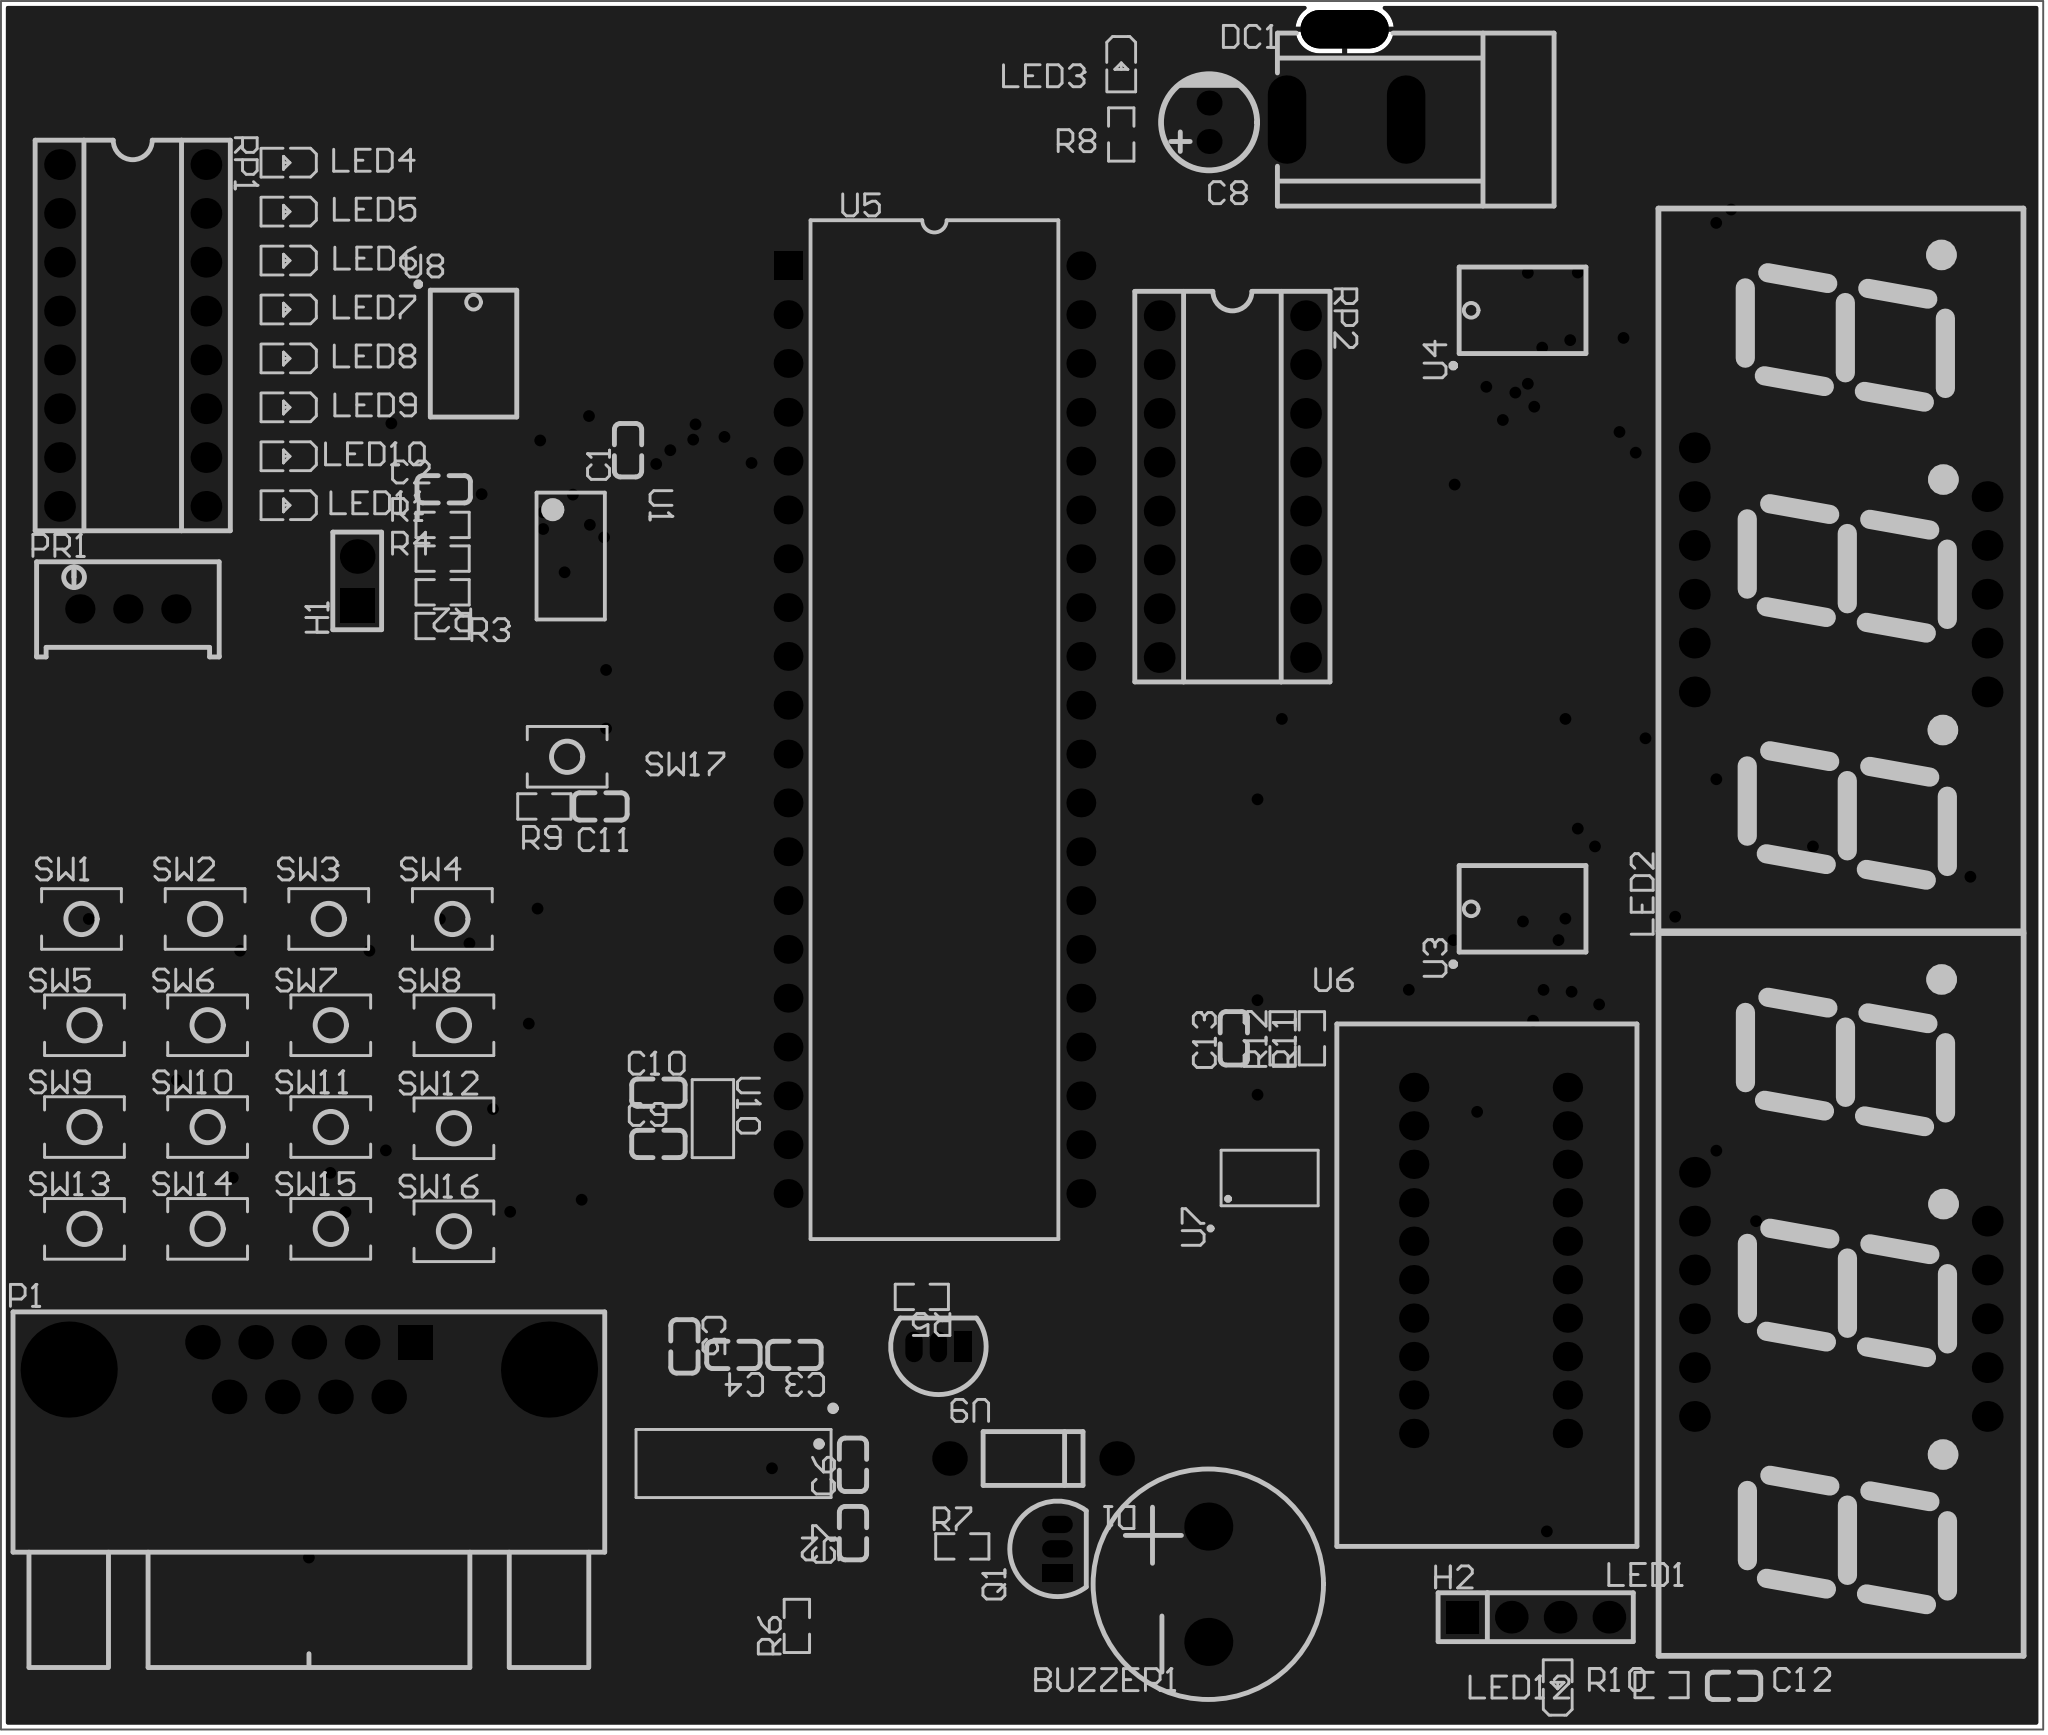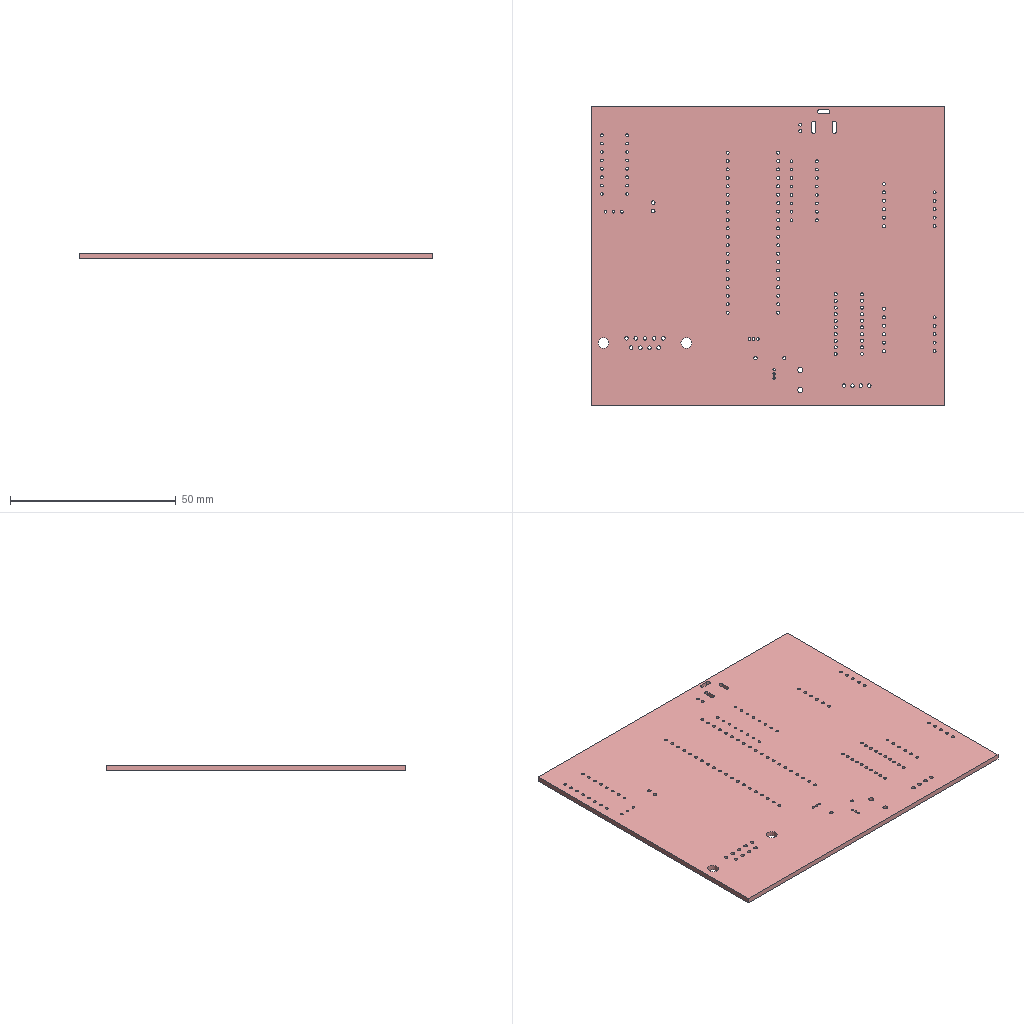Circuit board layout | Altium Designer | box 106.3 x 89.9 x 1.6 mm
Layer stack:
# Altium Designer layer stack of  (unit mm; dielectric type: 0 none, 1 core, 2 prepreg, 3 surface material)
index,name,kind,layer,copper_thickness_mm,dielectric_type,dielectric_thickness_mm,dielectric_material,dielectric_constant
0,Top Paste Mask Layer,other,,,,,,
1,Top Silkscreen Layer,other,,,,,,
2,Top Solder Mask Layer,dielectric,,,3,0.01,,3.3
3,Top Layer,copper,Top Layer,0.035,,,,
4,Dielectric1,dielectric,,,3,1.51,FR4,4.5
5,Bottom Layer,copper,Bottom Layer,0.035,,,,
6,Bottom Solder Mask Layer,dielectric,,,3,0.01,,3.3
7,Bottom Silkscreen Layer,other,,,,,,
8,Bottom Paste Mask Layer,other,,,,,,
# drill layer pairs: low layer,high layer
drill_pair,Top Layer,Bottom Layer
Part placement:
Designator,Comment,Layer,Footprint,Center-X(mm),Center-Y(mm),Rotation
BUZZER1,buzzer,TopLayer,BUZ-TH_BD12.0-P6.00-D0.9-RD,147.931,100.139,90
C1,104,TopLayer,C0603,117.729,159.131,90
C2,104,TopLayer,C0603,108.133,157.099,0
C3,104,TopLayer,C0603,126.389,112.069,180
C4,104,TopLayer,C0603,123.214,112.069,180
C5,104,TopLayer,C0603,120.664,112.512,270
C6,104,TopLayer,C0603,129.437,106.354,90
C7,104,TopLayer,C0603,129.437,102.798,90
C8,100uF,TopLayer,CAP-TH_BD5.0-P2.00-D0.8-FD-10UF50VC110GL,147.973,176.19,90
C9,20PF,TopLayer,C0603,119.31,123.044,0
C10,20PF,TopLayer,C0603,119.31,125.711,0
C11,10uF,TopLayer,C0603,116.293,140.6,0
C12,104,TopLayer,C0603,175.297,94.854,0
C13,104,TopLayer,C0603,149.26,128.538,90
D1,,TopLayer,DO_1N4007,138.811,106.68,180
DC1,,TopLayer,DC-005_2.5,155.129,178.682,0
H1,,TopLayer,HDR-TH_2P-P2.54-V-M-1,103.632,152.333,90
H2,,TopLayer,HDR-TH_4P-P2.54-V-M,164.973,98.425,0
LED1,3631BS,TopLayer,LED-SEG-TH_11P-L37.5-W19.0-P2.54-LS15.2-BL_1,180.856,115.219,90
LED2,3631BS,TopLayer,LED-SEG-TH_11P-L37.5-W19.0-P2.54-LS15.2-BL_1,180.848,152.908,90
LED3,,TopLayer,LED_0603,143.393,179.162,270
LED4,,TopLayer,LED_0603,100.015,174.095,180
LED5,,TopLayer,LED_0603,100.015,171.55,180
LED6,,TopLayer,LED_0603,100.015,169.004,180
LED7,,TopLayer,LED_0603,100.015,166.459,180
LED8,,TopLayer,LED_0603,100.015,163.913,180
LED9,,TopLayer,LED_0603,100.015,161.368,180
LED10,,TopLayer,LED_0603,100.015,158.822,180
LED11,,TopLayer,LED_0603,100.015,156.276,180
LED12,,TopLayer,LED_0603,166.124,94.818,90
P1,DB9FL,TopLayer,DB9-TH_DB9F,101.116,111.307,0
PR1,10kΩ,TopLayer,R_3296,91.694,150.876,0
Q1,,TopLayer,S8550P_TO-92,140.081,101.981,90
R1,10K,TopLayer,R0603,108.077,155.246,0
R2,1K,TopLayer,R0603,108.077,151.74,180
R3,1K,TopLayer,R0603,108.077,149.987,0
R4,510K,TopLayer,R0603,108.077,153.493,0
R5,4.7K,TopLayer,R0603,133.02,115.088,180
R6,0,TopLayer,R0603,126.516,97.972,90
R7,2K,TopLayer,R0603,135.128,102.108,0
R8,1K,TopLayer,R0603,143.401,175.555,270
R9,10K,TopLayer,R0603,113.372,140.6,0
R10,0,TopLayer,R0603,171.524,94.895,0
R11,4.7K,TopLayer,R0603,153.324,128.538,90
R12,4.7K,TopLayer,R0603,151.8,128.538,90
RP1,,TopLayer,DIP-16_L20.3-W10.2-P2.54-LS7.6-BL,91.948,165.1,270
RP2,,TopLayer,DIP-16_L20.3-W10.2-P2.54-LS7.6-BL,149.186,157.237,270
SW1,,TopLayer,Key_SMD_3x4x2,89.281,134.747,180
SW2,,TopLayer,Key_SMD_3x4x2,95.716,134.747,180
SW3,,TopLayer,Key_SMD_3x4x2,102.15,134.747,180
SW4,,TopLayer,Key_SMD_3x4x2,108.585,134.747,180
SW5,,TopLayer,Key_SMD_3x4x2,89.436,129.218,0
SW6,,TopLayer,Key_SMD_3x4x2,95.846,129.218,0
SW7,,TopLayer,Key_SMD_3x4x2,102.256,129.218,0
SW8,,TopLayer,Key_SMD_3x4x2,108.667,129.218,0
SW9,,TopLayer,Key_SMD_3x4x2,89.436,123.922,0
SW10,,TopLayer,Key_SMD_3x4x2,95.846,123.922,0
SW11,,TopLayer,Key_SMD_3x4x2,102.256,123.922,0
SW12,,TopLayer,Key_SMD_3x4x2,108.667,123.859,0
SW13,,TopLayer,Key_SMD_3x4x2,89.436,118.627,0
SW14,,TopLayer,Key_SMD_3x4x2,95.846,118.627,0
SW15,,TopLayer,Key_SMD_3x4x2,102.256,118.627,0
SW16,,TopLayer,Key_SMD_3x4x2,108.667,118.5,0
SW17,,TopLayer,Key_SMD_3x4x2,114.56,143.184,180
U1,ADC0804CN,TopLayer,ADC0804CN,114.745,153.626,270
U2,MAX232ESE,TopLayer,MAX232ESE,123.221,106.419,180
U3,MC74HC573DW,TopLayer,MC74HC573DW,164.239,135.295,90
U4,MC74HC573DW,TopLayer,MC74HC573DW,164.239,166.43,90
U5,P89C51RC2HBP,TopLayer,P89C51RC23N_01,133.678,144.595,270
U7,AT24C02,TopLayer,SOIC-8_L5.0-W4.0-P1.27-LS6.2-TL,151.124,121.272,90
U8,MC74HC573DW,TopLayer,MC74HC573DW,109.707,164.207,0
U9,DS18B20,TopLayer,TO-92-3_L4.9-W3.7-P1.27-L,133.884,112.489,180
U10,32768/10ppm/12.5pF,TopLayer,osc-smd_l3.2-w1.5,122.146,124.359,270
U6,DAC0832LCJ,TopLayer,DAC0832LCJ,162.624,116.984,0
Pad and via stacks:
# Altium Designer via and pad stacks of  (unit mm). Each distinct definition once, with the count of objects using it.
# via: kind,start_layer,end_layer,hole_mm,diameter_mm,mode(0 simple;1 top-mid-bottom;2 full stack),diameter_per_layer,count,example_net
# pad: kind,layer,hole_mm,hole_type(0 round;1 square;2 slot),plating,top_size,top_shape(1 round;2 rect;3 octagon;9 rounded rect),mid_size,bottom_size,mode,footprint,size_per_layer,count,example
pad,Multi-Layer,1.5,0,plated,2.5x2.5,1,2.5x2.5,2.5x2.5,0,BUZ-TH_BD12.0-P6.00-D0.9-RD,,2,BUZZER1.1
pad,Multi-Layer,0.9,0,plated,1.3x1.3,1,1.3x1.3,1.3x1.3,0,CAP-TH_BD5.0-P2.00-D0.8-FD-10UF50VC110GL,,2,C8.2
pad,Multi-Layer,1,0,plated,1.8x1.8,1,1.8x1.8,1.8x1.8,0,DO_1N4007,,2,D1.1
pad,Multi-Layer,1.2,2,plated,2x4.6,1,2x4.6,2x4.6,0,DC-005_2.5,,2,DC1.1
pad,Multi-Layer,1.2,2,plated,4.6x2,1,4.6x2,4.6x2,0,DC-005_2.5,,1,DC1.3
pad,Multi-Layer,1.1,0,plated,1.8x1.8,1,1.8x1.8,1.8x1.8,0,HDR-TH_2P-P2.54-V-M-1,,1,H1.2
pad,Multi-Layer,1.1,0,plated,1.8x1.8,2,1.8x1.8,1.8x1.8,0,HDR-TH_2P-P2.54-V-M-1,,1,H1.1
pad,Multi-Layer,1.1,0,plated,1.7x1.7,2,1.7x1.7,1.7x1.7,0,HDR-TH_4P-P2.54-V-M,,1,H2.1
pad,Multi-Layer,1.1,0,plated,1.7x1.7,1,1.7x1.7,1.7x1.7,0,HDR-TH_4P-P2.54-V-M,,3,H2.2
pad,Multi-Layer,0.9,0,plated,1.6x1.6,1,1.6x1.6,1.6x1.6,0,LED-SEG-TH_11P-L37.5-W19.0-P2.54-LS15.2-BL_1,,22,LED1.4
pad,Multi-Layer,3.25,0,plated,5x5,1,5x5,5x5,0,DB9-TH_DB9F,,2,P1.10
pad,Multi-Layer,1.1,0,plated,1.8x1.8,1,1.8x1.8,1.8x1.8,0,DB9-TH_DB9F,,8,P1.6
pad,Multi-Layer,1.1,0,plated,1.8x1.8,2,1.8x1.8,1.8x1.8,0,DB9-TH_DB9F,,1,P1.1
pad,Multi-Layer,0.762,0,plated,1.524x1.524,1,1.524x1.524,1.524x1.524,0,R_3296,,3,PR1.2
pad,Multi-Layer,0.7,0,plated,0.9x1.6,1,0.9x1.6,0.9x1.6,0,S8550P_TO-92,,2,Q1.3
pad,Multi-Layer,0.7,0,plated,0.9x1.6,2,0.9x1.6,0.9x1.6,0,S8550P_TO-92,,1,Q1.1
pad,Multi-Layer,0.8,0,plated,1.6x1.6,1,1.6x1.6,1.6x1.6,0,DIP-16_L20.3-W10.2-P2.54-LS7.6-BL,,32,RP1.1
pad,Multi-Layer,0.9,2,plated,1.5x1.5,1,1.5x1.5,1.5x1.5,0,P89C51RC23N_01,,39,U5.21
pad,Multi-Layer,0.9,2,plated,1.5x1.5,2,1.5x1.5,1.5x1.5,0,P89C51RC23N_01,,1,U5.1
pad,Multi-Layer,0.8,0,plated,0.9x1.6,1,0.9x1.6,0.9x1.6,0,TO-92-3_L4.9-W3.7-P1.27-L,,2,U9.3
pad,Multi-Layer,0.8,0,plated,0.9x1.6,2,0.9x1.6,0.9x1.6,0,TO-92-3_L4.9-W3.7-P1.27-L,,1,U9.1
pad,Multi-Layer,0.9144,0,plated,1.524x1.524,1,1.524x1.524,1.524x1.524,0,DAC0832LCJ,,20,U6.1
pad,Top Layer,0,0,plated,0.8x0.9,2,0.8x0.9,0.8x0.9,0,C0603,,24,C1.2
pad,Top Layer,0,0,plated,0.8001x0.8001,2,0.8001x0.8001,0.8001x0.8001,0,LED_0603,,20,LED3.1
pad,Top Layer,0,0,plated,0.8065x0.864,2,0.8065x0.864,0.8065x0.864,0,R0603,,24,R1.2
pad,Top Layer,0,0,plated,1.53x1.36,2,1.53x1.36,1.53x1.36,0,Key_SMD_3x4x2,,34,SW1.1
pad,Top Layer,0,0,plated,0.4x1.95,1,0.4x1.95,0.4x1.95,0,ADC0804CN,,20,U1.11
pad,Top Layer,0,0,plated,0.56x1.745,1,0.56x1.745,0.56x1.745,0,MAX232ESE,,16,U2.9
pad,Top Layer,0,0,plated,1.26x0.36,1,1.26x0.36,1.26x0.36,0,MC74HC573DW,,60,U3.1
pad,Top Layer,0,0,plated,1.751x0.5887,2,1.751x0.5887,1.751x0.5887,0,SOIC-8_L5.0-W4.0-P1.27-LS6.2-TL,,8,U7.1
pad,Top Layer,0,0,plated,1.05x1.7,2,1.05x1.7,1.05x1.7,0,osc-smd_l3.2-w1.5,,2,U10.1
via,Top Layer,Bottom Layer,0.3048,0.6101,0,,52,INT0
via,Top Layer,Bottom Layer,0.3048,0.61,0,,24,GND
Copper pours:
name,layer,net,type(0 solid;1 hatched;2 none)
Top Layer-GND,Top Layer,GND,0
Bottom Layer-GND,Bottom Layer,GND,0
Design rules, without the lines most boards share:
# Altium Designer design rules of  (exported by Altium Designer, unit mm)
# columns: name | kind | enabled | priority | scope1 | scope2 | descriptor | typed fields (field=value)
creepage | 65 | enabled | 1 | All | All | Creepage Distance Constraint =(0mil) (All),(All) |
PWR | 2 | enabled | 2 | (InNet('VCC')) | All | Width Constraint (Min=10mil) (Max=100mil) (Preferred=30mil) ((InNet('VCC'))) |
copperThickness1oz_2 | 2 | enabled | 3 | All | All | Width Constraint (Min=10mil) (Max=100mil) (Preferred=10mil) (All) |